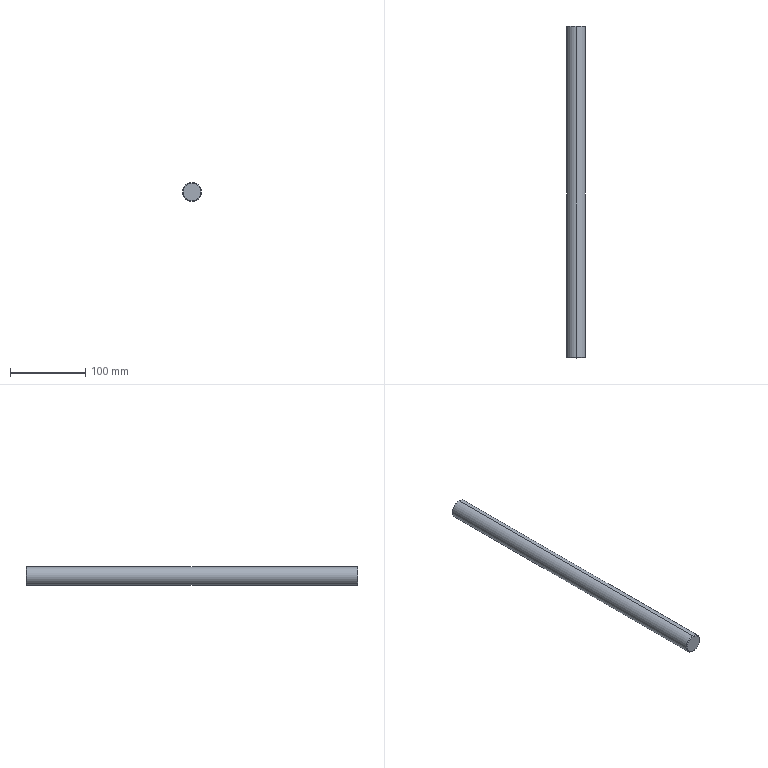Part | SolidWorks | features Chamfer 1, Extrusion 1, HoleWzd 1 | 1 solid | 12 faces | box 25 x 440 x 25 mm | volume 214356 mm3 | cone 6 | cylinder 4 | plane 2 | commonest cylinder face diameters 8.5 x2 25 x2
STEP:
#1=CARTESIAN_POINT('',(0.,413.5,-4.25));
#2=VERTEX_POINT('',#1);
#3=CARTESIAN_POINT('',(0.,413.5,4.25));
#4=VERTEX_POINT('',#3);
#5=CARTESIAN_POINT('',(0.,413.5,0.));
#6=DIRECTION('',(0.,1.,0.));
#7=DIRECTION('',(0.,0.,1.));
#8=AXIS2_PLACEMENT_3D('',#5,#6,#7);
#9=CIRCLE('',#8,4.25);
#10=EDGE_CURVE('',#2,#4,#9,.T.);
#11=ORIENTED_EDGE('',*,*,#10,.F.);
#12=CARTESIAN_POINT('',(0.,440.,-4.25));
#13=VERTEX_POINT('',#12);
#14=CARTESIAN_POINT('',(0.,440.,-4.25));
#15=DIRECTION('',(0.,1.,0.));
#16=VECTOR('',#15,1000.);
#17=LINE('',#14,#16);
#18=EDGE_CURVE('',#2,#13,#17,.T.);
#19=ORIENTED_EDGE('',*,*,#18,.T.);
#20=CARTESIAN_POINT('',(0.,440.,4.25));
#21=VERTEX_POINT('',#20);
#22=CARTESIAN_POINT('',(0.,440.,0.));
#23=DIRECTION('',(0.,1.,0.));
#24=DIRECTION('',(0.,0.,1.));
#25=AXIS2_PLACEMENT_3D('',#22,#23,#24);
#26=CIRCLE('',#25,4.25);
#27=EDGE_CURVE('',#13,#21,#26,.T.);
#28=ORIENTED_EDGE('',*,*,#27,.T.);
#29=CARTESIAN_POINT('',(0.,440.,4.25));
#30=DIRECTION('',(0.,1.,0.));
#31=VECTOR('',#30,1000.);
#32=LINE('',#29,#31);
#33=EDGE_CURVE('',#4,#21,#32,.T.);
#34=ORIENTED_EDGE('',*,*,#33,.F.);
#35=EDGE_LOOP('',(#11,#19,#28,#34));
#36=FACE_OUTER_BOUND('',#35,.T.);
#37=CARTESIAN_POINT('',(0.,440.,0.));
#38=DIRECTION('',(0.,1.,0.));
#39=DIRECTION('',(0.,0.,1.));
#40=AXIS2_PLACEMENT_3D('',#37,#38,#39);
#41=CYLINDRICAL_SURFACE('',#40,4.25);
#42=ADVANCED_FACE('',(#36),#41,.F.);
#43=CARTESIAN_POINT('',(0.,410.946,0.));
#44=VERTEX_POINT('',#43);
#45=CARTESIAN_POINT('',(0.,413.5,4.25));
#46=DIRECTION('',(0.,0.515,0.8572));
#47=VECTOR('',#46,1000.);
#48=LINE('',#45,#47);
#49=EDGE_CURVE('',#44,#4,#48,.T.);
#50=ORIENTED_EDGE('',*,*,#49,.F.);
#51=CARTESIAN_POINT('',(0.,413.5,-4.25));
#52=DIRECTION('',(0.,0.515,-0.8572));
#53=VECTOR('',#52,1000.);
#54=LINE('',#51,#53);
#55=EDGE_CURVE('',#44,#2,#54,.T.);
#56=ORIENTED_EDGE('',*,*,#55,.T.);
#57=ORIENTED_EDGE('',*,*,#10,.T.);
#58=EDGE_LOOP('',(#50,#56,#57));
#59=FACE_OUTER_BOUND('',#58,.T.);
#60=CARTESIAN_POINT('',(0.,413.5,0.));
#61=DIRECTION('',(0.,1.,0.));
#62=DIRECTION('',(0.,0.,1.));
#63=AXIS2_PLACEMENT_3D('',#60,#61,#62);
#64=CONICAL_SURFACE('',#63,4.25,1.03);
#65=ADVANCED_FACE('',(#59),#64,.F.);
#66=CARTESIAN_POINT('',(0.,440.,11.5));
#67=VERTEX_POINT('',#66);
#68=CARTESIAN_POINT('',(0.,440.,-11.5));
#69=VERTEX_POINT('',#68);
#70=CARTESIAN_POINT('',(0.,440.,0.));
#71=DIRECTION('',(0.,1.,0.));
#72=DIRECTION('',(0.,0.,1.));
#73=AXIS2_PLACEMENT_3D('',#70,#71,#72);
#74=CIRCLE('',#73,11.5);
#75=EDGE_CURVE('',#67,#69,#74,.T.);
#76=ORIENTED_EDGE('',*,*,#75,.F.);
#77=CARTESIAN_POINT('',(0.,439.,12.5));
#78=VERTEX_POINT('',#77);
#79=CARTESIAN_POINT('',(0.,440.,11.5));
#80=DIRECTION('',(0.,-0.7071,0.7071));
#81=VECTOR('',#80,1000.);
#82=LINE('',#79,#81);
#83=EDGE_CURVE('',#67,#78,#82,.T.);
#84=ORIENTED_EDGE('',*,*,#83,.T.);
#85=CARTESIAN_POINT('',(0.,439.,-12.5));
#86=VERTEX_POINT('',#85);
#87=CARTESIAN_POINT('',(0.,439.,0.));
#88=DIRECTION('',(0.,-1.,0.));
#89=DIRECTION('',(0.,0.,1.));
#90=AXIS2_PLACEMENT_3D('',#87,#88,#89);
#91=CIRCLE('',#90,12.5);
#92=EDGE_CURVE('',#86,#78,#91,.T.);
#93=ORIENTED_EDGE('',*,*,#92,.F.);
#94=CARTESIAN_POINT('',(0.,440.,-11.5));
#95=DIRECTION('',(0.,-0.7071,-0.7071));
#96=VECTOR('',#95,1000.);
#97=LINE('',#94,#96);
#98=EDGE_CURVE('',#69,#86,#97,.T.);
#99=ORIENTED_EDGE('',*,*,#98,.F.);
#100=EDGE_LOOP('',(#76,#84,#93,#99));
#101=FACE_OUTER_BOUND('',#100,.T.);
#102=CARTESIAN_POINT('',(0.,440.,0.));
#103=DIRECTION('',(0.,-1.,0.));
#104=DIRECTION('',(0.,0.,-1.));
#105=AXIS2_PLACEMENT_3D('',#102,#103,#104);
#106=CONICAL_SURFACE('',#105,11.5,0.7854);
#107=ADVANCED_FACE('',(#101),#106,.T.);
#108=CARTESIAN_POINT('',(0.,0.,-11.5));
#109=VERTEX_POINT('',#108);
#110=CARTESIAN_POINT('',(0.,0.,11.5));
#111=VERTEX_POINT('',#110);
#112=CARTESIAN_POINT('',(0.,0.,0.));
#113=DIRECTION('',(0.,-1.,0.));
#114=DIRECTION('',(0.,0.,1.));
#115=AXIS2_PLACEMENT_3D('',#112,#113,#114);
#116=CIRCLE('',#115,11.5);
#117=EDGE_CURVE('',#109,#111,#116,.T.);
#118=ORIENTED_EDGE('',*,*,#117,.F.);
#119=CARTESIAN_POINT('',(0.,1.,-12.5));
#120=VERTEX_POINT('',#119);
#121=CARTESIAN_POINT('',(0.,1.,-12.5));
#122=DIRECTION('',(0.,0.7071,-0.7071));
#123=VECTOR('',#122,1000.);
#124=LINE('',#121,#123);
#125=EDGE_CURVE('',#109,#120,#124,.T.);
#126=ORIENTED_EDGE('',*,*,#125,.T.);
#127=CARTESIAN_POINT('',(0.,1.,12.5));
#128=VERTEX_POINT('',#127);
#129=CARTESIAN_POINT('',(0.,1.,0.));
#130=DIRECTION('',(0.,1.,0.));
#131=DIRECTION('',(0.,0.,1.));
#132=AXIS2_PLACEMENT_3D('',#129,#130,#131);
#133=CIRCLE('',#132,12.5);
#134=EDGE_CURVE('',#128,#120,#133,.T.);
#135=ORIENTED_EDGE('',*,*,#134,.F.);
#136=CARTESIAN_POINT('',(0.,1.,12.5));
#137=DIRECTION('',(0.,0.7071,0.7071));
#138=VECTOR('',#137,1000.);
#139=LINE('',#136,#138);
#140=EDGE_CURVE('',#111,#128,#139,.T.);
#141=ORIENTED_EDGE('',*,*,#140,.F.);
#142=EDGE_LOOP('',(#118,#126,#135,#141));
#143=FACE_OUTER_BOUND('',#142,.T.);
#144=CARTESIAN_POINT('',(0.,1.,0.));
#145=DIRECTION('',(0.,1.,0.));
#146=DIRECTION('',(0.,0.,1.));
#147=AXIS2_PLACEMENT_3D('',#144,#145,#146);
#148=CONICAL_SURFACE('',#147,12.5,0.7854);
#149=ADVANCED_FACE('',(#143),#148,.T.);
#150=ORIENTED_EDGE('',*,*,#92,.T.);
#151=CARTESIAN_POINT('',(0.,440.,12.5));
#152=DIRECTION('',(0.,-1.,0.));
#153=VECTOR('',#152,1000.);
#154=LINE('',#151,#153);
#155=EDGE_CURVE('',#78,#128,#154,.T.);
#156=ORIENTED_EDGE('',*,*,#155,.T.);
#157=ORIENTED_EDGE('',*,*,#134,.T.);
#158=CARTESIAN_POINT('',(0.,440.,-12.5));
#159=DIRECTION('',(0.,-1.,0.));
#160=VECTOR('',#159,1000.);
#161=LINE('',#158,#160);
#162=EDGE_CURVE('',#86,#120,#161,.T.);
#163=ORIENTED_EDGE('',*,*,#162,.F.);
#164=EDGE_LOOP('',(#150,#156,#157,#163));
#165=FACE_OUTER_BOUND('',#164,.T.);
#166=CARTESIAN_POINT('',(0.,440.,0.));
#167=DIRECTION('',(0.,-1.,0.));
#168=DIRECTION('',(0.,0.,-1.));
#169=AXIS2_PLACEMENT_3D('',#166,#167,#168);
#170=CYLINDRICAL_SURFACE('',#169,12.5);
#171=ADVANCED_FACE('',(#165),#170,.T.);
#172=ORIENTED_EDGE('',*,*,#155,.F.);
#173=CARTESIAN_POINT('',(0.,439.,0.));
#174=DIRECTION('',(0.,-1.,0.));
#175=DIRECTION('',(0.,0.,1.));
#176=AXIS2_PLACEMENT_3D('',#173,#174,#175);
#177=CIRCLE('',#176,12.5);
#178=EDGE_CURVE('',#78,#86,#177,.T.);
#179=ORIENTED_EDGE('',*,*,#178,.T.);
#180=ORIENTED_EDGE('',*,*,#162,.T.);
#181=CARTESIAN_POINT('',(0.,1.,0.));
#182=DIRECTION('',(0.,1.,0.));
#183=DIRECTION('',(0.,0.,1.));
#184=AXIS2_PLACEMENT_3D('',#181,#182,#183);
#185=CIRCLE('',#184,12.5);
#186=EDGE_CURVE('',#120,#128,#185,.T.);
#187=ORIENTED_EDGE('',*,*,#186,.T.);
#188=EDGE_LOOP('',(#172,#179,#180,#187));
#189=FACE_OUTER_BOUND('',#188,.T.);
#190=CARTESIAN_POINT('',(0.,440.,0.));
#191=DIRECTION('',(0.,-1.,0.));
#192=DIRECTION('',(0.,0.,-1.));
#193=AXIS2_PLACEMENT_3D('',#190,#191,#192);
#194=CYLINDRICAL_SURFACE('',#193,12.5);
#195=ADVANCED_FACE('',(#189),#194,.T.);
#196=CARTESIAN_POINT('',(0.,440.,0.));
#197=DIRECTION('',(0.,1.,0.));
#198=DIRECTION('',(0.,0.,1.));
#199=AXIS2_PLACEMENT_3D('',#196,#197,#198);
#200=CIRCLE('',#199,4.25);
#201=EDGE_CURVE('',#21,#13,#200,.T.);
#202=ORIENTED_EDGE('',*,*,#201,.F.);
#203=ORIENTED_EDGE('',*,*,#27,.F.);
#204=EDGE_LOOP('',(#202,#203));
#205=FACE_BOUND('',#204,.T.);
#206=CARTESIAN_POINT('',(0.,440.,0.));
#207=DIRECTION('',(0.,1.,0.));
#208=DIRECTION('',(0.,0.,1.));
#209=AXIS2_PLACEMENT_3D('',#206,#207,#208);
#210=CIRCLE('',#209,11.5);
#211=EDGE_CURVE('',#69,#67,#210,.T.);
#212=ORIENTED_EDGE('',*,*,#211,.T.);
#213=ORIENTED_EDGE('',*,*,#75,.T.);
#214=EDGE_LOOP('',(#212,#213));
#215=FACE_OUTER_BOUND('',#214,.T.);
#216=CARTESIAN_POINT('',(0.,440.,0.));
#217=DIRECTION('',(0.,1.,0.));
#218=DIRECTION('',(0.,0.,1.));
#219=AXIS2_PLACEMENT_3D('',#216,#217,#218);
#220=PLANE('',#219);
#221=ADVANCED_FACE('',(#205,#215),#220,.T.);
#222=CARTESIAN_POINT('',(0.,0.,0.));
#223=DIRECTION('',(0.,-1.,0.));
#224=DIRECTION('',(0.,0.,1.));
#225=AXIS2_PLACEMENT_3D('',#222,#223,#224);
#226=CIRCLE('',#225,11.5);
#227=EDGE_CURVE('',#111,#109,#226,.T.);
#228=ORIENTED_EDGE('',*,*,#227,.T.);
#229=ORIENTED_EDGE('',*,*,#117,.T.);
#230=EDGE_LOOP('',(#228,#229));
#231=FACE_OUTER_BOUND('',#230,.T.);
#232=CARTESIAN_POINT('',(0.,0.,0.));
#233=DIRECTION('',(0.,1.,0.));
#234=DIRECTION('',(0.,0.,1.));
#235=AXIS2_PLACEMENT_3D('',#232,#233,#234);
#236=PLANE('',#235);
#237=ADVANCED_FACE('',(#231),#236,.F.);
#238=ORIENTED_EDGE('',*,*,#125,.F.);
#239=ORIENTED_EDGE('',*,*,#227,.F.);
#240=ORIENTED_EDGE('',*,*,#140,.T.);
#241=ORIENTED_EDGE('',*,*,#186,.F.);
#242=EDGE_LOOP('',(#238,#239,#240,#241));
#243=FACE_OUTER_BOUND('',#242,.T.);
#244=CARTESIAN_POINT('',(0.,1.,0.));
#245=DIRECTION('',(0.,1.,0.));
#246=DIRECTION('',(0.,0.,1.));
#247=AXIS2_PLACEMENT_3D('',#244,#245,#246);
#248=CONICAL_SURFACE('',#247,12.5,0.7854);
#249=ADVANCED_FACE('',(#243),#248,.T.);
#250=ORIENTED_EDGE('',*,*,#83,.F.);
#251=ORIENTED_EDGE('',*,*,#211,.F.);
#252=ORIENTED_EDGE('',*,*,#98,.T.);
#253=ORIENTED_EDGE('',*,*,#178,.F.);
#254=EDGE_LOOP('',(#250,#251,#252,#253));
#255=FACE_OUTER_BOUND('',#254,.T.);
#256=CARTESIAN_POINT('',(0.,440.,0.));
#257=DIRECTION('',(0.,-1.,0.));
#258=DIRECTION('',(0.,0.,-1.));
#259=AXIS2_PLACEMENT_3D('',#256,#257,#258);
#260=CONICAL_SURFACE('',#259,11.5,0.7854);
#261=ADVANCED_FACE('',(#255),#260,.T.);
#262=ORIENTED_EDGE('',*,*,#55,.F.);
#263=ORIENTED_EDGE('',*,*,#49,.T.);
#264=CARTESIAN_POINT('',(0.,413.5,0.));
#265=DIRECTION('',(0.,1.,0.));
#266=DIRECTION('',(0.,0.,1.));
#267=AXIS2_PLACEMENT_3D('',#264,#265,#266);
#268=CIRCLE('',#267,4.25);
#269=EDGE_CURVE('',#4,#2,#268,.T.);
#270=ORIENTED_EDGE('',*,*,#269,.T.);
#271=EDGE_LOOP('',(#262,#263,#270));
#272=FACE_OUTER_BOUND('',#271,.T.);
#273=CARTESIAN_POINT('',(0.,413.5,0.));
#274=DIRECTION('',(0.,1.,0.));
#275=DIRECTION('',(0.,0.,1.));
#276=AXIS2_PLACEMENT_3D('',#273,#274,#275);
#277=CONICAL_SURFACE('',#276,4.25,1.03);
#278=ADVANCED_FACE('',(#272),#277,.F.);
#279=ORIENTED_EDGE('',*,*,#18,.F.);
#280=ORIENTED_EDGE('',*,*,#269,.F.);
#281=ORIENTED_EDGE('',*,*,#33,.T.);
#282=ORIENTED_EDGE('',*,*,#201,.T.);
#283=EDGE_LOOP('',(#279,#280,#281,#282));
#284=FACE_OUTER_BOUND('',#283,.T.);
#285=CARTESIAN_POINT('',(0.,440.,0.));
#286=DIRECTION('',(0.,1.,0.));
#287=DIRECTION('',(0.,0.,1.));
#288=AXIS2_PLACEMENT_3D('',#285,#286,#287);
#289=CYLINDRICAL_SURFACE('',#288,4.25);
#290=ADVANCED_FACE('',(#284),#289,.F.);
#291=CLOSED_SHELL('',(#42,#65,#107,#149,#171,#195,#221,#237,#249,#261,#278,#290));
#292=MANIFOLD_SOLID_BREP('',#291);
#293=CARTESIAN_POINT('',(0.,0.,0.));
#294=DIRECTION('',(0.,0.,1.));
#295=DIRECTION('',(1.,0.,0.));
#296=AXIS2_PLACEMENT_3D('',#293,#294,#295);
#297=(LENGTH_UNIT()NAMED_UNIT(*)SI_UNIT(.MILLI.,.METRE.));
#298=UNCERTAINTY_MEASURE_WITH_UNIT(LENGTH_MEASURE(0.00001),#297,'','');
#299=(NAMED_UNIT(*)PLANE_ANGLE_UNIT()SI_UNIT($,.RADIAN.));
#300=(NAMED_UNIT(*)SI_UNIT($,.STERADIAN.)SOLID_ANGLE_UNIT());
#301=(GEOMETRIC_REPRESENTATION_CONTEXT(3)GLOBAL_UNCERTAINTY_ASSIGNED_CONTEXT((#298))GLOBAL_UNIT_ASSIGNED_CONTEXT((#297,#299,#300))REPRESENTATION_CONTEXT('',''));
#302=ADVANCED_BREP_SHAPE_REPRESENTATION('',(#292,#296),#301);